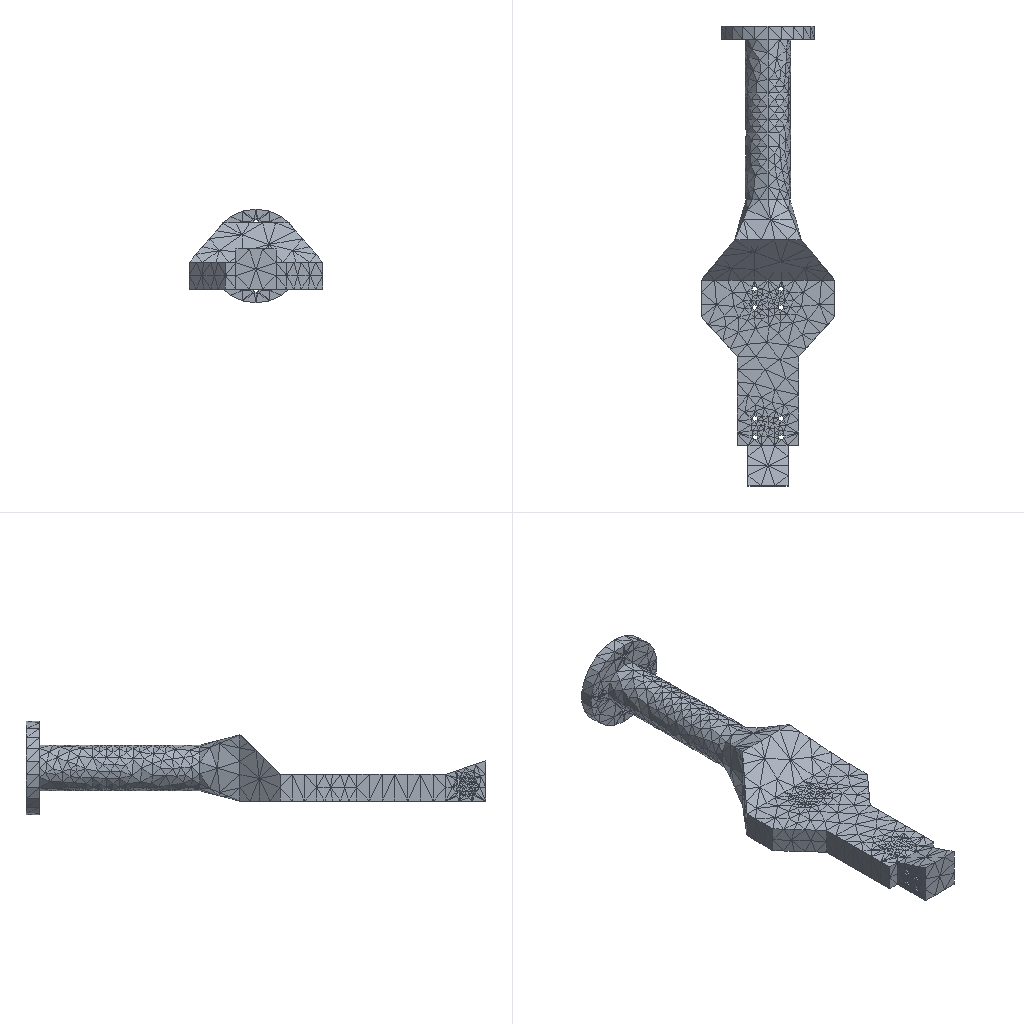Simulation study | ansys workbench
Ansys APDL input file, long lists of numbers shortened:
/batch
/config,noeldb,1     ! force off writing results to database
*get,_wallstrt,active,,time,wall
! ANSYS input file written by Workbench version 2022 R1
! File used for geometry attach:
/title,wbnew--____ (B5)
! ****** Begin Custom Load Command Snippet ******
/COM, ACT Extensions:
/COM,     LSDYNA, 2021.1
/COM,
! ****** End   Custom Load Command Snippet ******
*DIM,_wb_ProjectScratch_dir,string,248
_wb_ProjectScratch_dir(1) = ''
*DIM,_wb_SolverFiles_dir,string,248
_wb_SolverFiles_dir(1) = ''
*DIM,_wb_userfiles_dir,string,248
_wb_userfiles_dir(1) = ''
/com,--- Data in consistent NMM units. See Solving Units in the help system for more information.
/units,MPA
/nopr
/wb,file,start              !  signify a WB generated input file
/prep7
! Turn off shape checking because checks already performed inside WB mesher.
! See help system for more information.
SHPP,OFF,,NOWARN
/nolist
etcon,set             ! allow ANSYS to choose best KEYOP's for 180x elements, resets any applicable keyopt to MAPDL defaults
/com,*********** Nodes for the whole assembly ***********
nblock,3,,17708
(1i9,3e20.9e3)
        1    -1.464338266E+01    -3.140000000E+02    -2.084873734E+01
! (16098 more lines like these left out)
-1
/com,*********** Nodes for all Remote Points ***********
nblock,3
(1i9,3e20.9e3)
    16100     5.912518453E-05    -1.004697405E+02    -2.911433507E+00
-1
/wb,elem,start            !  set before creation of elements
/com,*********** Elements for Body 1 "__1-FreeParts|__2" ***********
et,1,187
eblock,19,solid,,9087
(19i9)
        1        1        1        1        0        0        0        0       10        0        1     1793     2543     1821     2509    13236    13383    13233    13235
! (18173 more lines like these left out)
-1
/wb,elem,end               !  done creating elements
/com,*********** Send User Defined Coordinate System(s) ***********
csys,0
toffst,273.15,  ! Temperature offset from absolute zero
/com,*********** Set Reference Temperature ***********
tref,22.
/wb,mat,start              !  starting to send materials
/com,*********** Send Materials ***********
Temperature = 'TEMP' ! Temperature
MP,DENS,1,7.85e-09,	! tonne mm^-3
MP,ALPX,1,1.2e-05,	! C^-1
MP,C,1,434000000,	! mm^2 s^-2 C^-1
MP,KXX,1,60.5,	! tonne mm s^-3 C^-1
MP,RSVX,1,0.00017,	! ohm mm
MP,EX,1,200000,	! tonne s^-2 mm^-1
MP,NUXY,1,0.3,
MP,MURX,1,10000,
/wb,mat,end                !  done sending materials
!************************* Model Summary ********************
!__1-FreeParts|__2,	结构钢,	matid,	1
!************************* End Model Summary ********************
! get the diagonal of the bounding box. Needed later for other things
*get,_xmin,node,,mnloc,x
*get,_ymin,node,,mnloc,y
*get,_zmin,node,,mnloc,z
*get,_xmax,node,,mxloc,x
*get,_ymax,node,,mxloc,y
*get,_zmax,node,,mxloc,z
_ASMDIAG=(_xmax-_xmin)*(_xmax-_xmin)+(_ymax-_ymin)*(_ymax-_ymin)+(_zmax-_zmin)*(_zmax-_zmin)
_ASMDIAG=SQRT(_ASMDIAG)
/wb,contact,start          !  starting to send contact
/wb,contact,end            !  done creating contacts
/com,*********** Send Named Selection as Node Component ***********
CMBLOCK,______  ,NODE,     1424
(8i10)
       105       106       107       108       113       114       115       116
! (177 more lines like these left out)
/golist
/wb,load,start             !  starting to send loads
/com,*********** Fixed Supports ***********
CMBLOCK,_FIXEDSU,NODE,     1424
(8i10)
       105       106       107       108       113       114       115       116
! (177 more lines like these left out)
cmsel,s,_FIXEDSU
d,all,all
nsel,all
/com,*********** Create Remote Point "内部远程点" ***********
! -------- Remote Point Used by "力矩" --------
*set,tid,3
*set,cid,2
et,cid,174
et,tid,170
keyo,tid,2,1               ! Don't fix the pilot node
keyo,tid,4,111111
keyo,cid,12,5              ! Bonded Contact
keyo,cid,4,1               ! Deformable RBE3 style load
keyo,cid,2,2               ! MPC style contact
eblock,10,,,798
(15i9)
    12891        2        2        2        0      248      249     1268     1268     4450     4459     1268     4452
! (797 more lines like these left out)
-1
*set,_npilot,16100
_npilot35=_npilot
type,tid
mat ,cid
real,cid
tshape,pilo
en,13689,_npilot
tshape
/com,*********** Construct Moment Using Remote Attachment ***********
/gst,on,on
fini
*get,_numnode,node,0,count
*get,_numelem,elem,0,count
*get, _MAXELEMNUM, elem, 0, NUM, MAX
*get, _MAXNODENUM, node, 0, NUM, MAX
*get, _MAXELEMTYPE, etyp, 0, NUM, MAX
*get, _MAXREALCONST, real, 0, NUM, MAX
/go
/wb,load,end               !  done creating loads
/com,--- Number of total nodes = %_numnode%
/com,--- Number of contact elements = 798
/com,--- Number of spring elements = 0
/com,--- Number of bearing elements = 0
/com,--- Number of solid elements = 9087
/com,--- Number of condensed parts = 0
/com,--- Number of total elements = %_numelem%
*get,_wallbsol,active,,time,wall
/com,****************************************************************************
/com,*************************    SOLUTION       ********************************
/com,****************************************************************************
/solu
antype,0                   ! static analysis
_thickRatio=  1     ! Ratio of thick parts in the model
eqsl,pcg,1e-8,,,,,,1
cntr,print,1               ! print out contact info and also make no initial contact an error
dmpoption,emat,no             ! Don't combine emat file for DANSYS
dmpoption,esav,no             ! Don't combine esav file for DANSYS
nldiag,cont,iter           ! print out contact info each equilibrium iteration
rescontrol,,none                 ! Do not keep any restart files
/com,****************************************************
/com,******************* SOLVE FOR LS 1 OF 1 ****************
nsel,s,node,,16100
f,all,mx,0.
f,all,my,520000.
f,all,mz,0.
nsel,all
/nopr
/gopr
nsub,1,1,1
time,1.
outres,erase
outres,all,none
outres,nsol,all,
outres,rsol,all
outres,eangl,all
outres,etmp,all
outres,veng,all
outres,strs,all,
outres,epel,all,
outres,eppl,all,
outres,cont,all,
! *********** WB SOLVE COMMAND ***********
! check interactive state
*get,ANSINTER_,active,,int
*if,ANSINTER_,ne,0,then
/eof
*endif
solve
/com *************** Write FE CONNECTORS *********
CEWRITE,file,ce,,INTE
/com,****************************************************
/com,*************** FINISHED SOLVE FOR LS 1 *************
*get,_wallasol,active,,time,wall
/nopr
*get,_numnode,node,0,count
*get,_numelem,elem,0,count
*get, _MAXELEMNUM, elem, 0, NUM, MAX
*get, _MAXNODENUM, node, 0, NUM, MAX,,,INTERNAL
*get, _MAXELEMTYPE, etyp, 0, NUM, MAX
*get, _MAXREALCONST, real, 0, NUM, MAX
/gopr
*get,_PCGITER,active,,solu,cgiter
/post1
xmlo,ENCODING,ISO-8859-1
xmlo,parm
/xml,parm,xml
fini
/gopr
*get,_walldone,active,,time,wall
_preptime=(_wallbsol-_wallstrt)*3600
_solvtime=(_wallasol-_wallbsol)*3600
_posttime=(_walldone-_wallasol)*3600
_totaltim=(_walldone-_wallstrt)*3600
*get,_dlbratio,active,0,solu,dlbr
*get,_combtime,active,0,solu,comb
*get,_ssmode,active,0,solu,ssmm
*get,_ndofs,active,0,solu,ndof
*get,_sol_end_time,active,0,set,time
*if,_sol_end_time,eq,1.,then
/fclean				!clean distributed files
*endif
/com,--- Total number of nodes = %_numnode%
/com,--- Total number of elements = %_numelem%
/com,--- Element load balance ratio = %_dlbratio%
/com,--- Time to combine distributed files = %_combtime%
/com,--- Sparse memory mode = %_ssmode%
/com,--- Number of DOF = %_ndofs%
/wb,file,end               ! done with WB generated input